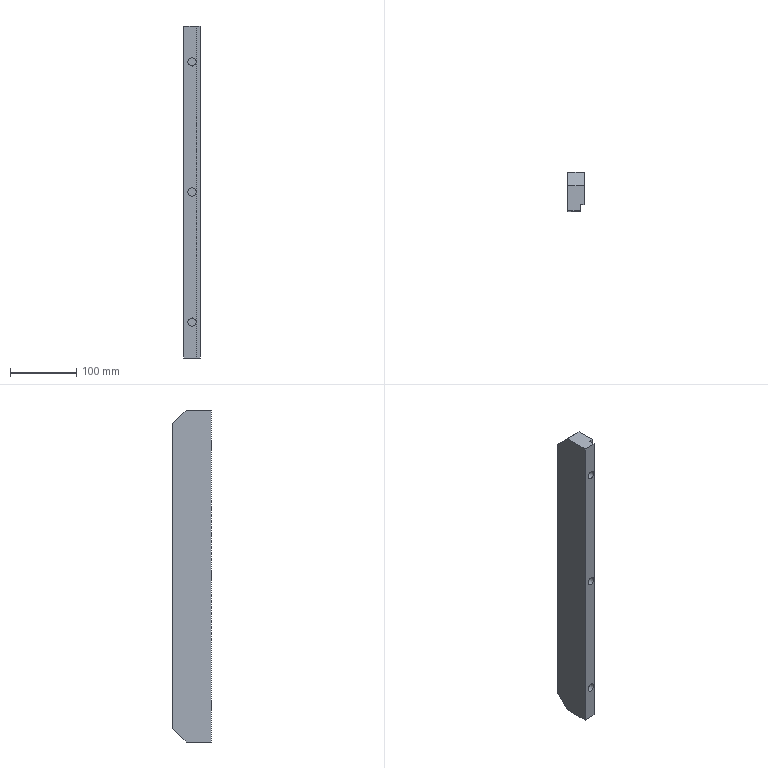CAM job | NX | 3-axis milling, drilling | part box 25 x 58 x 500 mm | stock box 25 x 58 x 505 mm
Tools:
number,name,description,diameter,corner_radius,flute_length,length,flutes
1,ZXZ,Milling Tool-5 Parameters,6.0,0.0,50.0,75.0,2
3,12.5ZT,Drilling Tool,12.5,0.0,35.0,50.0,2
7,D6A45,Milling Tool-5 Parameters,6.0,0.0,3.0,3.0,2
2,D26R0.8,Milling Tool-5 Parameters,26.0,0.8,50.0,75.0,2
11,D10JING,Milling Tool-5 Parameters,10.0,0.0,50.0,75.0,2
Operations:
program,operation,operation_type,tool,method,geometry_group,spindle_rpm,surface_speed,feed_per_tooth,feed_cut,feed_plunge,cut_length_mm,path_length_mm,cut_time_min,machine_time_min
1,FLOOR_WALL,VolumeBased25DMillingOperation,D26R0.8,METHOD,A,1500.0,122.0,0.6667,2000.0,100.0,8070.0,16258.0,4.035,4.854
1,ZLEVEL_PROFILE,ZLevelMilling,D26R0.8,METHOD,A,1800.0,147.0,0.6111,2200.0,100.0,8671.16,8750.478,3.941,3.949
1,DRILLING_COPY,Operation,12.5ZT,METHOD,A,800.0,31.0,0.075,120.0,0.0,119.266,696.578,0.9939,1.052
1,FLOOR_WALL_1,VolumeBased25DMillingOperation,D10JING,METHOD,A,5000.0,157.0,0.125,1250.0,100.0,522.0,596.0,0.4176,0.425
1,ZLEVEL_PROFILE_COPY_1_COPY_COPY_COPY,ZLevelMilling,D6A45,METHOD,A,7000.0,131.0,0.0714,1000.0,1000.0,1158.972,2247.314,1.159,1.268
1,ZLEVEL_PROFILE_COPY_1_COPY_COPY_COPY_COPY,ZLevelMilling,D6A45,METHOD,A,7000.0,131.0,0.0714,1000.0,1000.0,511.219,593.219,0.5112,0.5194
PROGRAM_COPY,DRILLING,Operation,ZXZ,METHOD,A,3000.0,56.0,0.0333,200.0,0.0,12.0,678.034,0.06,0.1266